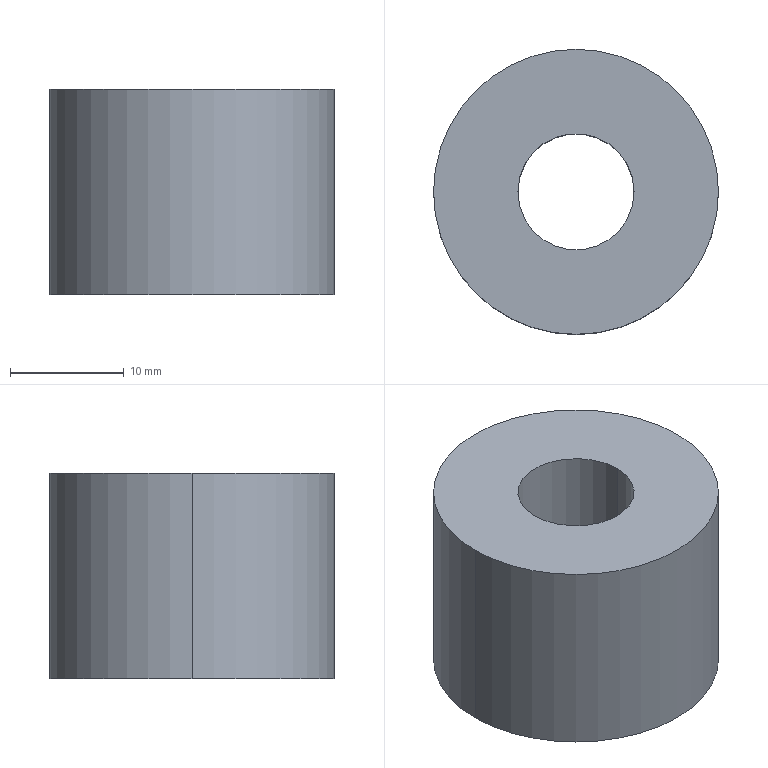Part | SolidWorks | features Extrusion 1, HoleWzd 1 | 1 solid | 6 faces | box 25 x 25 x 18 mm | volume 7365 mm3 | cylinder 4 | plane 2 | commonest cylinder face diameters 10.2 x2 25 x2
STEP:
#1=CARTESIAN_POINT('',(-5.1,0.,0.));
#2=VERTEX_POINT('',#1);
#3=CARTESIAN_POINT('',(5.1,0.,0.));
#4=VERTEX_POINT('',#3);
#5=CARTESIAN_POINT('',(0.,0.,0.));
#6=DIRECTION('',(0.,0.,1.));
#7=DIRECTION('',(1.,0.,0.));
#8=AXIS2_PLACEMENT_3D('',#5,#6,#7);
#9=CIRCLE('',#8,5.1);
#10=EDGE_CURVE('',#2,#4,#9,.T.);
#11=ORIENTED_EDGE('',*,*,#10,.F.);
#12=CARTESIAN_POINT('',(-5.1,0.,18.));
#13=VERTEX_POINT('',#12);
#14=CARTESIAN_POINT('',(-5.1,0.,18.));
#15=DIRECTION('',(0.,0.,1.));
#16=VECTOR('',#15,1000.);
#17=LINE('',#14,#16);
#18=EDGE_CURVE('',#2,#13,#17,.T.);
#19=ORIENTED_EDGE('',*,*,#18,.T.);
#20=CARTESIAN_POINT('',(5.1,0.,18.));
#21=VERTEX_POINT('',#20);
#22=CARTESIAN_POINT('',(0.,0.,18.));
#23=DIRECTION('',(0.,0.,1.));
#24=DIRECTION('',(1.,0.,0.));
#25=AXIS2_PLACEMENT_3D('',#22,#23,#24);
#26=CIRCLE('',#25,5.1);
#27=EDGE_CURVE('',#13,#21,#26,.T.);
#28=ORIENTED_EDGE('',*,*,#27,.T.);
#29=CARTESIAN_POINT('',(5.1,0.,18.));
#30=DIRECTION('',(0.,0.,1.));
#31=VECTOR('',#30,1000.);
#32=LINE('',#29,#31);
#33=EDGE_CURVE('',#4,#21,#32,.T.);
#34=ORIENTED_EDGE('',*,*,#33,.F.);
#35=EDGE_LOOP('',(#11,#19,#28,#34));
#36=FACE_OUTER_BOUND('',#35,.T.);
#37=CARTESIAN_POINT('',(0.,0.,18.));
#38=DIRECTION('',(0.,0.,1.));
#39=DIRECTION('',(1.,0.,0.));
#40=AXIS2_PLACEMENT_3D('',#37,#38,#39);
#41=CYLINDRICAL_SURFACE('',#40,5.1);
#42=ADVANCED_FACE('',(#36),#41,.F.);
#43=CARTESIAN_POINT('',(12.5,0.,18.));
#44=VERTEX_POINT('',#43);
#45=CARTESIAN_POINT('',(-12.5,0.,18.));
#46=VERTEX_POINT('',#45);
#47=CARTESIAN_POINT('',(0.,0.,18.));
#48=DIRECTION('',(0.,0.,1.));
#49=DIRECTION('',(1.,0.,0.));
#50=AXIS2_PLACEMENT_3D('',#47,#48,#49);
#51=CIRCLE('',#50,12.5);
#52=EDGE_CURVE('',#44,#46,#51,.T.);
#53=ORIENTED_EDGE('',*,*,#52,.F.);
#54=CARTESIAN_POINT('',(12.5,0.,0.));
#55=VERTEX_POINT('',#54);
#56=CARTESIAN_POINT('',(12.5,0.,18.));
#57=DIRECTION('',(0.,0.,-1.));
#58=VECTOR('',#57,1000.);
#59=LINE('',#56,#58);
#60=EDGE_CURVE('',#44,#55,#59,.T.);
#61=ORIENTED_EDGE('',*,*,#60,.T.);
#62=CARTESIAN_POINT('',(-12.5,0.,0.));
#63=VERTEX_POINT('',#62);
#64=CARTESIAN_POINT('',(0.,0.,0.));
#65=DIRECTION('',(0.,0.,1.));
#66=DIRECTION('',(1.,0.,0.));
#67=AXIS2_PLACEMENT_3D('',#64,#65,#66);
#68=CIRCLE('',#67,12.5);
#69=EDGE_CURVE('',#55,#63,#68,.T.);
#70=ORIENTED_EDGE('',*,*,#69,.T.);
#71=CARTESIAN_POINT('',(-12.5,0.,18.));
#72=DIRECTION('',(0.,0.,-1.));
#73=VECTOR('',#72,1000.);
#74=LINE('',#71,#73);
#75=EDGE_CURVE('',#46,#63,#74,.T.);
#76=ORIENTED_EDGE('',*,*,#75,.F.);
#77=EDGE_LOOP('',(#53,#61,#70,#76));
#78=FACE_OUTER_BOUND('',#77,.T.);
#79=CARTESIAN_POINT('',(0.,0.,18.));
#80=DIRECTION('',(0.,0.,-1.));
#81=DIRECTION('',(-1.,0.,0.));
#82=AXIS2_PLACEMENT_3D('',#79,#80,#81);
#83=CYLINDRICAL_SURFACE('',#82,12.5);
#84=ADVANCED_FACE('',(#78),#83,.T.);
#85=ORIENTED_EDGE('',*,*,#60,.F.);
#86=CARTESIAN_POINT('',(0.,0.,18.));
#87=DIRECTION('',(0.,0.,1.));
#88=DIRECTION('',(1.,0.,0.));
#89=AXIS2_PLACEMENT_3D('',#86,#87,#88);
#90=CIRCLE('',#89,12.5);
#91=EDGE_CURVE('',#46,#44,#90,.T.);
#92=ORIENTED_EDGE('',*,*,#91,.F.);
#93=ORIENTED_EDGE('',*,*,#75,.T.);
#94=CARTESIAN_POINT('',(0.,0.,0.));
#95=DIRECTION('',(0.,0.,1.));
#96=DIRECTION('',(1.,0.,0.));
#97=AXIS2_PLACEMENT_3D('',#94,#95,#96);
#98=CIRCLE('',#97,12.5);
#99=EDGE_CURVE('',#63,#55,#98,.T.);
#100=ORIENTED_EDGE('',*,*,#99,.T.);
#101=EDGE_LOOP('',(#85,#92,#93,#100));
#102=FACE_OUTER_BOUND('',#101,.T.);
#103=CARTESIAN_POINT('',(0.,0.,18.));
#104=DIRECTION('',(0.,0.,-1.));
#105=DIRECTION('',(-1.,0.,0.));
#106=AXIS2_PLACEMENT_3D('',#103,#104,#105);
#107=CYLINDRICAL_SURFACE('',#106,12.5);
#108=ADVANCED_FACE('',(#102),#107,.T.);
#109=CARTESIAN_POINT('',(0.,0.,18.));
#110=DIRECTION('',(0.,0.,1.));
#111=DIRECTION('',(1.,0.,0.));
#112=AXIS2_PLACEMENT_3D('',#109,#110,#111);
#113=CIRCLE('',#112,5.1);
#114=EDGE_CURVE('',#21,#13,#113,.T.);
#115=ORIENTED_EDGE('',*,*,#114,.F.);
#116=ORIENTED_EDGE('',*,*,#27,.F.);
#117=EDGE_LOOP('',(#115,#116));
#118=FACE_BOUND('',#117,.T.);
#119=ORIENTED_EDGE('',*,*,#91,.T.);
#120=ORIENTED_EDGE('',*,*,#52,.T.);
#121=EDGE_LOOP('',(#119,#120));
#122=FACE_OUTER_BOUND('',#121,.T.);
#123=CARTESIAN_POINT('',(0.,0.,18.));
#124=DIRECTION('',(0.,0.,1.));
#125=DIRECTION('',(1.,0.,0.));
#126=AXIS2_PLACEMENT_3D('',#123,#124,#125);
#127=PLANE('',#126);
#128=ADVANCED_FACE('',(#118,#122),#127,.T.);
#129=CARTESIAN_POINT('',(0.,0.,0.));
#130=DIRECTION('',(0.,0.,1.));
#131=DIRECTION('',(1.,0.,0.));
#132=AXIS2_PLACEMENT_3D('',#129,#130,#131);
#133=CIRCLE('',#132,5.1);
#134=EDGE_CURVE('',#4,#2,#133,.T.);
#135=ORIENTED_EDGE('',*,*,#134,.T.);
#136=ORIENTED_EDGE('',*,*,#10,.T.);
#137=EDGE_LOOP('',(#135,#136));
#138=FACE_BOUND('',#137,.T.);
#139=ORIENTED_EDGE('',*,*,#99,.F.);
#140=ORIENTED_EDGE('',*,*,#69,.F.);
#141=EDGE_LOOP('',(#139,#140));
#142=FACE_OUTER_BOUND('',#141,.T.);
#143=CARTESIAN_POINT('',(0.,0.,0.));
#144=DIRECTION('',(0.,0.,1.));
#145=DIRECTION('',(1.,0.,0.));
#146=AXIS2_PLACEMENT_3D('',#143,#144,#145);
#147=PLANE('',#146);
#148=ADVANCED_FACE('',(#138,#142),#147,.F.);
#149=ORIENTED_EDGE('',*,*,#18,.F.);
#150=ORIENTED_EDGE('',*,*,#134,.F.);
#151=ORIENTED_EDGE('',*,*,#33,.T.);
#152=ORIENTED_EDGE('',*,*,#114,.T.);
#153=EDGE_LOOP('',(#149,#150,#151,#152));
#154=FACE_OUTER_BOUND('',#153,.T.);
#155=CARTESIAN_POINT('',(0.,0.,18.));
#156=DIRECTION('',(0.,0.,1.));
#157=DIRECTION('',(1.,0.,0.));
#158=AXIS2_PLACEMENT_3D('',#155,#156,#157);
#159=CYLINDRICAL_SURFACE('',#158,5.1);
#160=ADVANCED_FACE('',(#154),#159,.F.);
#161=CLOSED_SHELL('',(#42,#84,#108,#128,#148,#160));
#162=MANIFOLD_SOLID_BREP('',#161);
#163=CARTESIAN_POINT('',(0.,0.,0.));
#164=DIRECTION('',(0.,0.,1.));
#165=DIRECTION('',(1.,0.,0.));
#166=AXIS2_PLACEMENT_3D('',#163,#164,#165);
#167=(LENGTH_UNIT()NAMED_UNIT(*)SI_UNIT(.MILLI.,.METRE.));
#168=UNCERTAINTY_MEASURE_WITH_UNIT(LENGTH_MEASURE(0.00001),#167,'','');
#169=(NAMED_UNIT(*)PLANE_ANGLE_UNIT()SI_UNIT($,.RADIAN.));
#170=(NAMED_UNIT(*)SI_UNIT($,.STERADIAN.)SOLID_ANGLE_UNIT());
#171=(GEOMETRIC_REPRESENTATION_CONTEXT(3)GLOBAL_UNCERTAINTY_ASSIGNED_CONTEXT((#168))GLOBAL_UNIT_ASSIGNED_CONTEXT((#167,#169,#170))REPRESENTATION_CONTEXT('',''));
#172=ADVANCED_BREP_SHAPE_REPRESENTATION('',(#162,#166),#171);